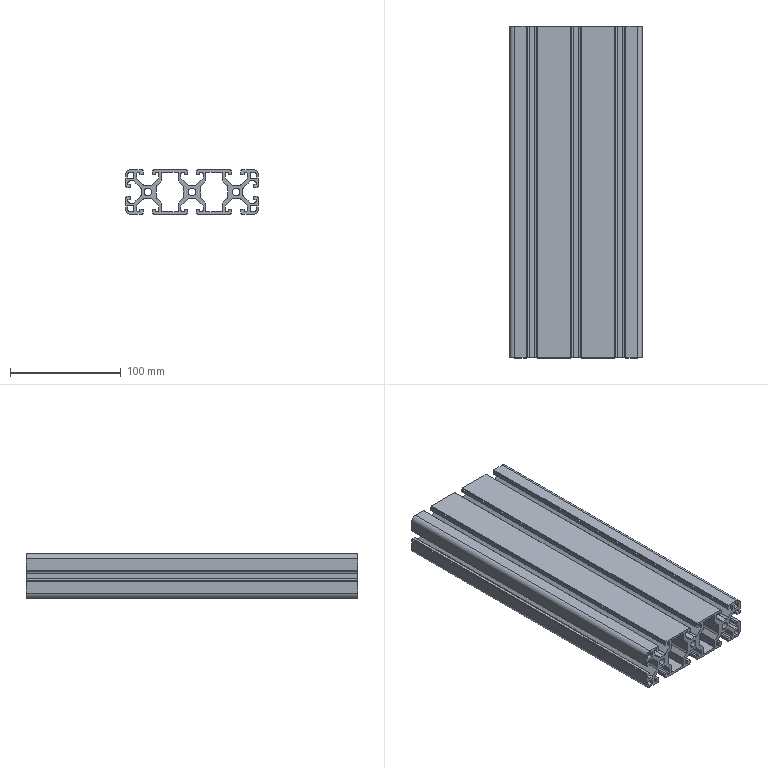Part | STEP file | Handling mechanism support_Default<machined> | 1 solid | 260 faces | box 120 x 300 x 40 mm | volume 478423 mm3 | plane 190 | cylinder 70 | commonest cylinder face diameters 6 x24 4 x20 2 x16 6.8 x6 9 x4